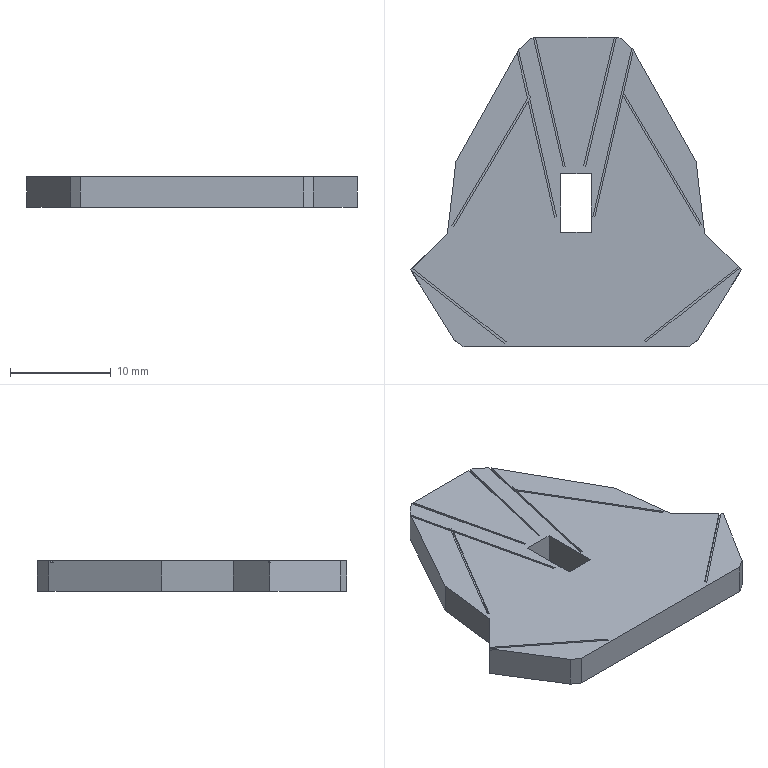Part | SolidWorks | features BaseBody 1 | 1 solid | 57 faces | box 32.817 x 30.753 x 3 mm | volume 2054 mm3 | plane 45 | spline 12